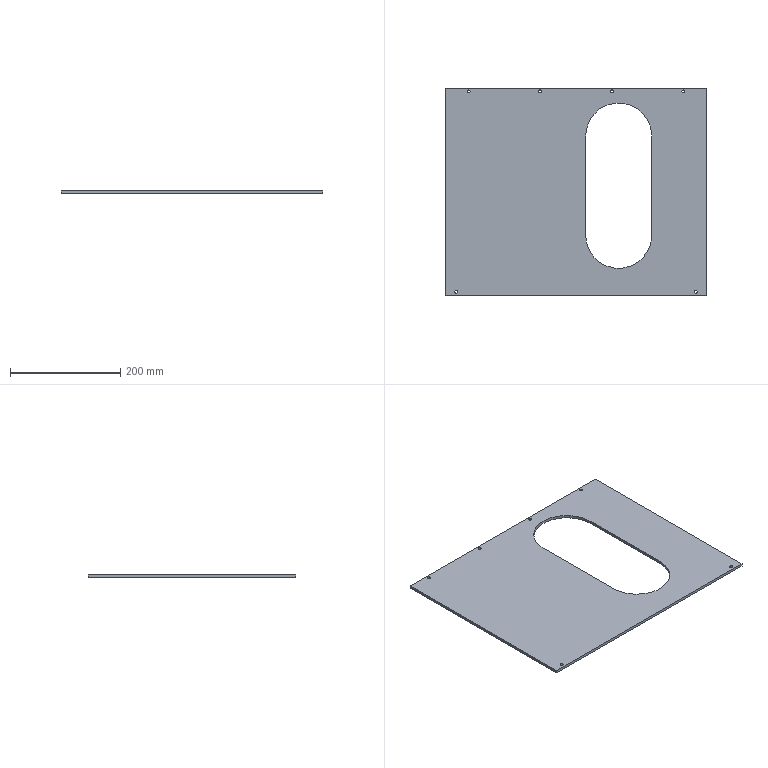Part | SolidWorks | features Extrusion 1, HoleWzd 1, ICE 1 | 1 solid | 22 faces | box 475 x 377 x 5 mm | volume 730114 mm3 | cylinder 14 | plane 8 | commonest cylinder face diameters 5.5 x12 120 x2
STEP:
#1=CARTESIAN_POINT('',(192.25,182.5,5.));
#2=VERTEX_POINT('',#1);
#3=CARTESIAN_POINT('',(197.75,182.5,5.));
#4=VERTEX_POINT('',#3);
#5=CARTESIAN_POINT('',(195.,182.5,5.));
#6=DIRECTION('',(0.,0.,1.));
#7=DIRECTION('',(1.,0.,0.));
#8=AXIS2_PLACEMENT_3D('',#5,#6,#7);
#9=CIRCLE('',#8,2.75);
#10=EDGE_CURVE('',#2,#4,#9,.T.);
#11=ORIENTED_EDGE('',*,*,#10,.T.);
#12=CARTESIAN_POINT('',(197.75,182.5,0.));
#13=VERTEX_POINT('',#12);
#14=CARTESIAN_POINT('',(197.75,182.5,0.));
#15=DIRECTION('',(0.,0.,-1.));
#16=VECTOR('',#15,1000.);
#17=LINE('',#14,#16);
#18=EDGE_CURVE('',#4,#13,#17,.T.);
#19=ORIENTED_EDGE('',*,*,#18,.T.);
#20=CARTESIAN_POINT('',(192.25,182.5,0.));
#21=VERTEX_POINT('',#20);
#22=CARTESIAN_POINT('',(195.,182.5,0.));
#23=DIRECTION('',(0.,0.,-1.));
#24=DIRECTION('',(-1.,0.,0.));
#25=AXIS2_PLACEMENT_3D('',#22,#23,#24);
#26=CIRCLE('',#25,2.75);
#27=EDGE_CURVE('',#13,#21,#26,.T.);
#28=ORIENTED_EDGE('',*,*,#27,.T.);
#29=CARTESIAN_POINT('',(192.25,182.5,0.));
#30=DIRECTION('',(0.,0.,-1.));
#31=VECTOR('',#30,1000.);
#32=LINE('',#29,#31);
#33=EDGE_CURVE('',#2,#21,#32,.T.);
#34=ORIENTED_EDGE('',*,*,#33,.F.);
#35=EDGE_LOOP('',(#11,#19,#28,#34));
#36=FACE_OUTER_BOUND('',#35,.T.);
#37=CARTESIAN_POINT('',(195.,182.5,0.));
#38=DIRECTION('',(0.,0.,-1.));
#39=DIRECTION('',(-1.,0.,0.));
#40=AXIS2_PLACEMENT_3D('',#37,#38,#39);
#41=CYLINDRICAL_SURFACE('',#40,2.75);
#42=ADVANCED_FACE('',(#36),#41,.F.);
#43=CARTESIAN_POINT('',(62.25,182.5,5.));
#44=VERTEX_POINT('',#43);
#45=CARTESIAN_POINT('',(67.75,182.5,5.));
#46=VERTEX_POINT('',#45);
#47=CARTESIAN_POINT('',(65.,182.5,5.));
#48=DIRECTION('',(0.,0.,1.));
#49=DIRECTION('',(1.,0.,0.));
#50=AXIS2_PLACEMENT_3D('',#47,#48,#49);
#51=CIRCLE('',#50,2.75);
#52=EDGE_CURVE('',#44,#46,#51,.T.);
#53=ORIENTED_EDGE('',*,*,#52,.T.);
#54=CARTESIAN_POINT('',(67.75,182.5,0.));
#55=VERTEX_POINT('',#54);
#56=CARTESIAN_POINT('',(67.75,182.5,0.));
#57=DIRECTION('',(0.,0.,-1.));
#58=VECTOR('',#57,1000.);
#59=LINE('',#56,#58);
#60=EDGE_CURVE('',#46,#55,#59,.T.);
#61=ORIENTED_EDGE('',*,*,#60,.T.);
#62=CARTESIAN_POINT('',(62.25,182.5,0.));
#63=VERTEX_POINT('',#62);
#64=CARTESIAN_POINT('',(65.,182.5,0.));
#65=DIRECTION('',(0.,0.,-1.));
#66=DIRECTION('',(-1.,0.,0.));
#67=AXIS2_PLACEMENT_3D('',#64,#65,#66);
#68=CIRCLE('',#67,2.75);
#69=EDGE_CURVE('',#55,#63,#68,.T.);
#70=ORIENTED_EDGE('',*,*,#69,.T.);
#71=CARTESIAN_POINT('',(62.25,182.5,0.));
#72=DIRECTION('',(0.,0.,-1.));
#73=VECTOR('',#72,1000.);
#74=LINE('',#71,#73);
#75=EDGE_CURVE('',#44,#63,#74,.T.);
#76=ORIENTED_EDGE('',*,*,#75,.F.);
#77=EDGE_LOOP('',(#53,#61,#70,#76));
#78=FACE_OUTER_BOUND('',#77,.T.);
#79=CARTESIAN_POINT('',(65.,182.5,0.));
#80=DIRECTION('',(0.,0.,-1.));
#81=DIRECTION('',(-1.,0.,0.));
#82=AXIS2_PLACEMENT_3D('',#79,#80,#81);
#83=CYLINDRICAL_SURFACE('',#82,2.75);
#84=ADVANCED_FACE('',(#78),#83,.F.);
#85=CARTESIAN_POINT('',(-67.75,182.5,5.));
#86=VERTEX_POINT('',#85);
#87=CARTESIAN_POINT('',(-62.25,182.5,5.));
#88=VERTEX_POINT('',#87);
#89=CARTESIAN_POINT('',(-65.,182.5,5.));
#90=DIRECTION('',(0.,0.,1.));
#91=DIRECTION('',(1.,0.,0.));
#92=AXIS2_PLACEMENT_3D('',#89,#90,#91);
#93=CIRCLE('',#92,2.75);
#94=EDGE_CURVE('',#86,#88,#93,.T.);
#95=ORIENTED_EDGE('',*,*,#94,.T.);
#96=CARTESIAN_POINT('',(-62.25,182.5,0.));
#97=VERTEX_POINT('',#96);
#98=CARTESIAN_POINT('',(-62.25,182.5,0.));
#99=DIRECTION('',(0.,0.,-1.));
#100=VECTOR('',#99,1000.);
#101=LINE('',#98,#100);
#102=EDGE_CURVE('',#88,#97,#101,.T.);
#103=ORIENTED_EDGE('',*,*,#102,.T.);
#104=CARTESIAN_POINT('',(-67.75,182.5,0.));
#105=VERTEX_POINT('',#104);
#106=CARTESIAN_POINT('',(-65.,182.5,0.));
#107=DIRECTION('',(0.,0.,-1.));
#108=DIRECTION('',(-1.,0.,0.));
#109=AXIS2_PLACEMENT_3D('',#106,#107,#108);
#110=CIRCLE('',#109,2.75);
#111=EDGE_CURVE('',#97,#105,#110,.T.);
#112=ORIENTED_EDGE('',*,*,#111,.T.);
#113=CARTESIAN_POINT('',(-67.75,182.5,0.));
#114=DIRECTION('',(0.,0.,-1.));
#115=VECTOR('',#114,1000.);
#116=LINE('',#113,#115);
#117=EDGE_CURVE('',#86,#105,#116,.T.);
#118=ORIENTED_EDGE('',*,*,#117,.F.);
#119=EDGE_LOOP('',(#95,#103,#112,#118));
#120=FACE_OUTER_BOUND('',#119,.T.);
#121=CARTESIAN_POINT('',(-65.,182.5,0.));
#122=DIRECTION('',(0.,0.,-1.));
#123=DIRECTION('',(-1.,0.,0.));
#124=AXIS2_PLACEMENT_3D('',#121,#122,#123);
#125=CYLINDRICAL_SURFACE('',#124,2.75);
#126=ADVANCED_FACE('',(#120),#125,.F.);
#127=CARTESIAN_POINT('',(-197.75,182.5,5.));
#128=VERTEX_POINT('',#127);
#129=CARTESIAN_POINT('',(-192.25,182.5,5.));
#130=VERTEX_POINT('',#129);
#131=CARTESIAN_POINT('',(-195.,182.5,5.));
#132=DIRECTION('',(0.,0.,1.));
#133=DIRECTION('',(1.,0.,0.));
#134=AXIS2_PLACEMENT_3D('',#131,#132,#133);
#135=CIRCLE('',#134,2.75);
#136=EDGE_CURVE('',#128,#130,#135,.T.);
#137=ORIENTED_EDGE('',*,*,#136,.T.);
#138=CARTESIAN_POINT('',(-192.25,182.5,0.));
#139=VERTEX_POINT('',#138);
#140=CARTESIAN_POINT('',(-192.25,182.5,0.));
#141=DIRECTION('',(0.,0.,-1.));
#142=VECTOR('',#141,1000.);
#143=LINE('',#140,#142);
#144=EDGE_CURVE('',#130,#139,#143,.T.);
#145=ORIENTED_EDGE('',*,*,#144,.T.);
#146=CARTESIAN_POINT('',(-197.75,182.5,0.));
#147=VERTEX_POINT('',#146);
#148=CARTESIAN_POINT('',(-195.,182.5,0.));
#149=DIRECTION('',(0.,0.,-1.));
#150=DIRECTION('',(-1.,0.,0.));
#151=AXIS2_PLACEMENT_3D('',#148,#149,#150);
#152=CIRCLE('',#151,2.75);
#153=EDGE_CURVE('',#139,#147,#152,.T.);
#154=ORIENTED_EDGE('',*,*,#153,.T.);
#155=CARTESIAN_POINT('',(-197.75,182.5,0.));
#156=DIRECTION('',(0.,0.,-1.));
#157=VECTOR('',#156,1000.);
#158=LINE('',#155,#157);
#159=EDGE_CURVE('',#128,#147,#158,.T.);
#160=ORIENTED_EDGE('',*,*,#159,.F.);
#161=EDGE_LOOP('',(#137,#145,#154,#160));
#162=FACE_OUTER_BOUND('',#161,.T.);
#163=CARTESIAN_POINT('',(-195.,182.5,0.));
#164=DIRECTION('',(0.,0.,-1.));
#165=DIRECTION('',(-1.,0.,0.));
#166=AXIS2_PLACEMENT_3D('',#163,#164,#165);
#167=CYLINDRICAL_SURFACE('',#166,2.75);
#168=ADVANCED_FACE('',(#162),#167,.F.);
#169=CARTESIAN_POINT('',(-220.25,-181.,5.));
#170=VERTEX_POINT('',#169);
#171=CARTESIAN_POINT('',(-214.75,-181.,5.));
#172=VERTEX_POINT('',#171);
#173=CARTESIAN_POINT('',(-217.5,-181.,5.));
#174=DIRECTION('',(0.,0.,1.));
#175=DIRECTION('',(1.,0.,0.));
#176=AXIS2_PLACEMENT_3D('',#173,#174,#175);
#177=CIRCLE('',#176,2.75);
#178=EDGE_CURVE('',#170,#172,#177,.T.);
#179=ORIENTED_EDGE('',*,*,#178,.T.);
#180=CARTESIAN_POINT('',(-214.75,-181.,0.));
#181=VERTEX_POINT('',#180);
#182=CARTESIAN_POINT('',(-214.75,-181.,0.));
#183=DIRECTION('',(0.,0.,-1.));
#184=VECTOR('',#183,1000.);
#185=LINE('',#182,#184);
#186=EDGE_CURVE('',#172,#181,#185,.T.);
#187=ORIENTED_EDGE('',*,*,#186,.T.);
#188=CARTESIAN_POINT('',(-220.25,-181.,0.));
#189=VERTEX_POINT('',#188);
#190=CARTESIAN_POINT('',(-217.5,-181.,0.));
#191=DIRECTION('',(0.,0.,-1.));
#192=DIRECTION('',(-1.,0.,0.));
#193=AXIS2_PLACEMENT_3D('',#190,#191,#192);
#194=CIRCLE('',#193,2.75);
#195=EDGE_CURVE('',#181,#189,#194,.T.);
#196=ORIENTED_EDGE('',*,*,#195,.T.);
#197=CARTESIAN_POINT('',(-220.25,-181.,0.));
#198=DIRECTION('',(0.,0.,-1.));
#199=VECTOR('',#198,1000.);
#200=LINE('',#197,#199);
#201=EDGE_CURVE('',#170,#189,#200,.T.);
#202=ORIENTED_EDGE('',*,*,#201,.F.);
#203=EDGE_LOOP('',(#179,#187,#196,#202));
#204=FACE_OUTER_BOUND('',#203,.T.);
#205=CARTESIAN_POINT('',(-217.5,-181.,0.));
#206=DIRECTION('',(0.,0.,-1.));
#207=DIRECTION('',(-1.,0.,0.));
#208=AXIS2_PLACEMENT_3D('',#205,#206,#207);
#209=CYLINDRICAL_SURFACE('',#208,2.75);
#210=ADVANCED_FACE('',(#204),#209,.F.);
#211=CARTESIAN_POINT('',(214.75,-181.,5.));
#212=VERTEX_POINT('',#211);
#213=CARTESIAN_POINT('',(220.25,-181.,5.));
#214=VERTEX_POINT('',#213);
#215=CARTESIAN_POINT('',(217.5,-181.,5.));
#216=DIRECTION('',(0.,0.,1.));
#217=DIRECTION('',(1.,0.,0.));
#218=AXIS2_PLACEMENT_3D('',#215,#216,#217);
#219=CIRCLE('',#218,2.75);
#220=EDGE_CURVE('',#212,#214,#219,.T.);
#221=ORIENTED_EDGE('',*,*,#220,.T.);
#222=CARTESIAN_POINT('',(220.25,-181.,0.));
#223=VERTEX_POINT('',#222);
#224=CARTESIAN_POINT('',(220.25,-181.,0.));
#225=DIRECTION('',(0.,0.,-1.));
#226=VECTOR('',#225,1000.);
#227=LINE('',#224,#226);
#228=EDGE_CURVE('',#214,#223,#227,.T.);
#229=ORIENTED_EDGE('',*,*,#228,.T.);
#230=CARTESIAN_POINT('',(214.75,-181.,0.));
#231=VERTEX_POINT('',#230);
#232=CARTESIAN_POINT('',(217.5,-181.,0.));
#233=DIRECTION('',(0.,0.,-1.));
#234=DIRECTION('',(-1.,0.,0.));
#235=AXIS2_PLACEMENT_3D('',#232,#233,#234);
#236=CIRCLE('',#235,2.75);
#237=EDGE_CURVE('',#223,#231,#236,.T.);
#238=ORIENTED_EDGE('',*,*,#237,.T.);
#239=CARTESIAN_POINT('',(214.75,-181.,0.));
#240=DIRECTION('',(0.,0.,-1.));
#241=VECTOR('',#240,1000.);
#242=LINE('',#239,#241);
#243=EDGE_CURVE('',#212,#231,#242,.T.);
#244=ORIENTED_EDGE('',*,*,#243,.F.);
#245=EDGE_LOOP('',(#221,#229,#238,#244));
#246=FACE_OUTER_BOUND('',#245,.T.);
#247=CARTESIAN_POINT('',(217.5,-181.,0.));
#248=DIRECTION('',(0.,0.,-1.));
#249=DIRECTION('',(-1.,0.,0.));
#250=AXIS2_PLACEMENT_3D('',#247,#248,#249);
#251=CYLINDRICAL_SURFACE('',#250,2.75);
#252=ADVANCED_FACE('',(#246),#251,.F.);
#253=CARTESIAN_POINT('',(137.5,101.5,0.));
#254=VERTEX_POINT('',#253);
#255=CARTESIAN_POINT('',(137.5,-78.5,0.));
#256=VERTEX_POINT('',#255);
#257=CARTESIAN_POINT('',(137.5,101.5,0.));
#258=DIRECTION('',(0.,-1.,0.));
#259=VECTOR('',#258,1000.);
#260=LINE('',#257,#259);
#261=EDGE_CURVE('',#254,#256,#260,.T.);
#262=ORIENTED_EDGE('',*,*,#261,.F.);
#263=CARTESIAN_POINT('',(17.5,101.5,0.));
#264=VERTEX_POINT('',#263);
#265=CARTESIAN_POINT('',(77.5,101.5,0.));
#266=DIRECTION('',(0.,0.,-1.));
#267=DIRECTION('',(-1.,0.,0.));
#268=AXIS2_PLACEMENT_3D('',#265,#266,#267);
#269=CIRCLE('',#268,60.);
#270=EDGE_CURVE('',#264,#254,#269,.T.);
#271=ORIENTED_EDGE('',*,*,#270,.F.);
#272=CARTESIAN_POINT('',(17.5,-78.5,0.));
#273=VERTEX_POINT('',#272);
#274=CARTESIAN_POINT('',(17.5,101.5,0.));
#275=DIRECTION('',(0.,1.,0.));
#276=VECTOR('',#275,1000.);
#277=LINE('',#274,#276);
#278=EDGE_CURVE('',#273,#264,#277,.T.);
#279=ORIENTED_EDGE('',*,*,#278,.F.);
#280=CARTESIAN_POINT('',(77.5,-78.5,0.));
#281=DIRECTION('',(0.,0.,-1.));
#282=DIRECTION('',(-1.,0.,0.));
#283=AXIS2_PLACEMENT_3D('',#280,#281,#282);
#284=CIRCLE('',#283,60.);
#285=EDGE_CURVE('',#256,#273,#284,.T.);
#286=ORIENTED_EDGE('',*,*,#285,.F.);
#287=EDGE_LOOP('',(#262,#271,#279,#286));
#288=FACE_BOUND('',#287,.T.);
#289=CARTESIAN_POINT('',(195.,182.5,0.));
#290=DIRECTION('',(0.,0.,-1.));
#291=DIRECTION('',(-1.,0.,0.));
#292=AXIS2_PLACEMENT_3D('',#289,#290,#291);
#293=CIRCLE('',#292,2.75);
#294=EDGE_CURVE('',#21,#13,#293,.T.);
#295=ORIENTED_EDGE('',*,*,#294,.F.);
#296=ORIENTED_EDGE('',*,*,#27,.F.);
#297=EDGE_LOOP('',(#295,#296));
#298=FACE_BOUND('',#297,.T.);
#299=CARTESIAN_POINT('',(65.,182.5,0.));
#300=DIRECTION('',(0.,0.,-1.));
#301=DIRECTION('',(-1.,0.,0.));
#302=AXIS2_PLACEMENT_3D('',#299,#300,#301);
#303=CIRCLE('',#302,2.75);
#304=EDGE_CURVE('',#63,#55,#303,.T.);
#305=ORIENTED_EDGE('',*,*,#304,.F.);
#306=ORIENTED_EDGE('',*,*,#69,.F.);
#307=EDGE_LOOP('',(#305,#306));
#308=FACE_BOUND('',#307,.T.);
#309=CARTESIAN_POINT('',(-195.,182.5,0.));
#310=DIRECTION('',(0.,0.,-1.));
#311=DIRECTION('',(-1.,0.,0.));
#312=AXIS2_PLACEMENT_3D('',#309,#310,#311);
#313=CIRCLE('',#312,2.75);
#314=EDGE_CURVE('',#147,#139,#313,.T.);
#315=ORIENTED_EDGE('',*,*,#314,.F.);
#316=ORIENTED_EDGE('',*,*,#153,.F.);
#317=EDGE_LOOP('',(#315,#316));
#318=FACE_BOUND('',#317,.T.);
#319=CARTESIAN_POINT('',(-217.5,-181.,0.));
#320=DIRECTION('',(0.,0.,-1.));
#321=DIRECTION('',(-1.,0.,0.));
#322=AXIS2_PLACEMENT_3D('',#319,#320,#321);
#323=CIRCLE('',#322,2.75);
#324=EDGE_CURVE('',#189,#181,#323,.T.);
#325=ORIENTED_EDGE('',*,*,#324,.F.);
#326=ORIENTED_EDGE('',*,*,#195,.F.);
#327=EDGE_LOOP('',(#325,#326));
#328=FACE_BOUND('',#327,.T.);
#329=CARTESIAN_POINT('',(217.5,-181.,0.));
#330=DIRECTION('',(0.,0.,-1.));
#331=DIRECTION('',(-1.,0.,0.));
#332=AXIS2_PLACEMENT_3D('',#329,#330,#331);
#333=CIRCLE('',#332,2.75);
#334=EDGE_CURVE('',#231,#223,#333,.T.);
#335=ORIENTED_EDGE('',*,*,#334,.F.);
#336=ORIENTED_EDGE('',*,*,#237,.F.);
#337=EDGE_LOOP('',(#335,#336));
#338=FACE_BOUND('',#337,.T.);
#339=CARTESIAN_POINT('',(237.5,-188.5,0.));
#340=VERTEX_POINT('',#339);
#341=CARTESIAN_POINT('',(237.5,188.5,0.));
#342=VERTEX_POINT('',#341);
#343=CARTESIAN_POINT('',(237.5,188.5,0.));
#344=DIRECTION('',(0.,1.,0.));
#345=VECTOR('',#344,1000.);
#346=LINE('',#343,#345);
#347=EDGE_CURVE('',#340,#342,#346,.T.);
#348=ORIENTED_EDGE('',*,*,#347,.F.);
#349=CARTESIAN_POINT('',(-237.5,-188.5,0.));
#350=VERTEX_POINT('',#349);
#351=CARTESIAN_POINT('',(-237.5,-188.5,0.));
#352=DIRECTION('',(1.,0.,0.));
#353=VECTOR('',#352,1000.);
#354=LINE('',#351,#353);
#355=EDGE_CURVE('',#350,#340,#354,.T.);
#356=ORIENTED_EDGE('',*,*,#355,.F.);
#357=CARTESIAN_POINT('',(-237.5,188.5,0.));
#358=VERTEX_POINT('',#357);
#359=CARTESIAN_POINT('',(-237.5,188.5,0.));
#360=DIRECTION('',(0.,-1.,0.));
#361=VECTOR('',#360,1000.);
#362=LINE('',#359,#361);
#363=EDGE_CURVE('',#358,#350,#362,.T.);
#364=ORIENTED_EDGE('',*,*,#363,.F.);
#365=CARTESIAN_POINT('',(-237.5,188.5,0.));
#366=DIRECTION('',(-1.,0.,0.));
#367=VECTOR('',#366,1000.);
#368=LINE('',#365,#367);
#369=EDGE_CURVE('',#342,#358,#368,.T.);
#370=ORIENTED_EDGE('',*,*,#369,.F.);
#371=EDGE_LOOP('',(#348,#356,#364,#370));
#372=FACE_OUTER_BOUND('',#371,.T.);
#373=CARTESIAN_POINT('',(-65.,182.5,0.));
#374=DIRECTION('',(0.,0.,-1.));
#375=DIRECTION('',(-1.,0.,0.));
#376=AXIS2_PLACEMENT_3D('',#373,#374,#375);
#377=CIRCLE('',#376,2.75);
#378=EDGE_CURVE('',#105,#97,#377,.T.);
#379=ORIENTED_EDGE('',*,*,#378,.F.);
#380=ORIENTED_EDGE('',*,*,#111,.F.);
#381=EDGE_LOOP('',(#379,#380));
#382=FACE_BOUND('',#381,.T.);
#383=CARTESIAN_POINT('',(0.,0.,0.));
#384=DIRECTION('',(0.,0.,1.));
#385=DIRECTION('',(1.,0.,0.));
#386=AXIS2_PLACEMENT_3D('',#383,#384,#385);
#387=PLANE('',#386);
#388=ADVANCED_FACE('',(#288,#298,#308,#318,#328,#338,#372,#382),#387,.F.);
#389=ORIENTED_EDGE('',*,*,#347,.T.);
#390=CARTESIAN_POINT('',(237.5,188.5,5.));
#391=VERTEX_POINT('',#390);
#392=CARTESIAN_POINT('',(237.5,188.5,5.));
#393=DIRECTION('',(0.,0.,-1.));
#394=VECTOR('',#393,1000.);
#395=LINE('',#392,#394);
#396=EDGE_CURVE('',#391,#342,#395,.T.);
#397=ORIENTED_EDGE('',*,*,#396,.F.);
#398=CARTESIAN_POINT('',(237.5,-188.5,5.));
#399=VERTEX_POINT('',#398);
#400=CARTESIAN_POINT('',(237.5,188.5,5.));
#401=DIRECTION('',(0.,1.,0.));
#402=VECTOR('',#401,1000.);
#403=LINE('',#400,#402);
#404=EDGE_CURVE('',#399,#391,#403,.T.);
#405=ORIENTED_EDGE('',*,*,#404,.F.);
#406=CARTESIAN_POINT('',(237.5,-188.5,5.));
#407=DIRECTION('',(0.,0.,-1.));
#408=VECTOR('',#407,1000.);
#409=LINE('',#406,#408);
#410=EDGE_CURVE('',#399,#340,#409,.T.);
#411=ORIENTED_EDGE('',*,*,#410,.T.);
#412=EDGE_LOOP('',(#389,#397,#405,#411));
#413=FACE_OUTER_BOUND('',#412,.T.);
#414=CARTESIAN_POINT('',(237.5,188.5,5.));
#415=DIRECTION('',(-1.,0.,0.));
#416=DIRECTION('',(0.,-1.,0.));
#417=AXIS2_PLACEMENT_3D('',#414,#415,#416);
#418=PLANE('',#417);
#419=ADVANCED_FACE('',(#413),#418,.F.);
#420=ORIENTED_EDGE('',*,*,#369,.T.);
#421=CARTESIAN_POINT('',(-237.5,188.5,5.));
#422=VERTEX_POINT('',#421);
#423=CARTESIAN_POINT('',(-237.5,188.5,5.));
#424=DIRECTION('',(0.,0.,-1.));
#425=VECTOR('',#424,1000.);
#426=LINE('',#423,#425);
#427=EDGE_CURVE('',#422,#358,#426,.T.);
#428=ORIENTED_EDGE('',*,*,#427,.F.);
#429=CARTESIAN_POINT('',(-237.5,188.5,5.));
#430=DIRECTION('',(-1.,0.,0.));
#431=VECTOR('',#430,1000.);
#432=LINE('',#429,#431);
#433=EDGE_CURVE('',#391,#422,#432,.T.);
#434=ORIENTED_EDGE('',*,*,#433,.F.);
#435=ORIENTED_EDGE('',*,*,#396,.T.);
#436=EDGE_LOOP('',(#420,#428,#434,#435));
#437=FACE_OUTER_BOUND('',#436,.T.);
#438=CARTESIAN_POINT('',(-237.5,188.5,5.));
#439=DIRECTION('',(0.,-1.,0.));
#440=DIRECTION('',(0.,0.,-1.));
#441=AXIS2_PLACEMENT_3D('',#438,#439,#440);
#442=PLANE('',#441);
#443=ADVANCED_FACE('',(#437),#442,.F.);
#444=ORIENTED_EDGE('',*,*,#363,.T.);
#445=CARTESIAN_POINT('',(-237.5,-188.5,5.));
#446=VERTEX_POINT('',#445);
#447=CARTESIAN_POINT('',(-237.5,-188.5,5.));
#448=DIRECTION('',(0.,0.,-1.));
#449=VECTOR('',#448,1000.);
#450=LINE('',#447,#449);
#451=EDGE_CURVE('',#446,#350,#450,.T.);
#452=ORIENTED_EDGE('',*,*,#451,.F.);
#453=CARTESIAN_POINT('',(-237.5,188.5,5.));
#454=DIRECTION('',(0.,-1.,0.));
#455=VECTOR('',#454,1000.);
#456=LINE('',#453,#455);
#457=EDGE_CURVE('',#422,#446,#456,.T.);
#458=ORIENTED_EDGE('',*,*,#457,.F.);
#459=ORIENTED_EDGE('',*,*,#427,.T.);
#460=EDGE_LOOP('',(#444,#452,#458,#459));
#461=FACE_OUTER_BOUND('',#460,.T.);
#462=CARTESIAN_POINT('',(-237.5,188.5,5.));
#463=DIRECTION('',(1.,0.,0.));
#464=DIRECTION('',(0.,0.,-1.));
#465=AXIS2_PLACEMENT_3D('',#462,#463,#464);
#466=PLANE('',#465);
#467=ADVANCED_FACE('',(#461),#466,.F.);
#468=ORIENTED_EDGE('',*,*,#355,.T.);
#469=ORIENTED_EDGE('',*,*,#410,.F.);
#470=CARTESIAN_POINT('',(-237.5,-188.5,5.));
#471=DIRECTION('',(1.,0.,0.));
#472=VECTOR('',#471,1000.);
#473=LINE('',#470,#472);
#474=EDGE_CURVE('',#446,#399,#473,.T.);
#475=ORIENTED_EDGE('',*,*,#474,.F.);
#476=ORIENTED_EDGE('',*,*,#451,.T.);
#477=EDGE_LOOP('',(#468,#469,#475,#476));
#478=FACE_OUTER_BOUND('',#477,.T.);
#479=CARTESIAN_POINT('',(-237.5,-188.5,5.));
#480=DIRECTION('',(0.,1.,0.));
#481=DIRECTION('',(0.,0.,1.));
#482=AXIS2_PLACEMENT_3D('',#479,#480,#481);
#483=PLANE('',#482);
#484=ADVANCED_FACE('',(#478),#483,.F.);
#485=CARTESIAN_POINT('',(137.5,101.5,5.));
#486=VERTEX_POINT('',#485);
#487=CARTESIAN_POINT('',(17.5,101.5,5.));
#488=VERTEX_POINT('',#487);
#489=CARTESIAN_POINT('',(77.5,101.5,5.));
#490=DIRECTION('',(0.,0.,1.));
#491=DIRECTION('',(1.,0.,0.));
#492=AXIS2_PLACEMENT_3D('',#489,#490,#491);
#493=CIRCLE('',#492,60.);
#494=EDGE_CURVE('',#486,#488,#493,.T.);
#495=ORIENTED_EDGE('',*,*,#494,.F.);
#496=CARTESIAN_POINT('',(137.5,-78.5,5.));
#497=VERTEX_POINT('',#496);
#498=CARTESIAN_POINT('',(137.5,0.,5.));
#499=DIRECTION('',(0.,1.,0.));
#500=VECTOR('',#499,1000.);
#501=LINE('',#498,#500);
#502=EDGE_CURVE('',#497,#486,#501,.T.);
#503=ORIENTED_EDGE('',*,*,#502,.F.);
#504=CARTESIAN_POINT('',(17.5,-78.5,5.));
#505=VERTEX_POINT('',#504);
#506=CARTESIAN_POINT('',(77.5,-78.5,5.));
#507=DIRECTION('',(0.,0.,1.));
#508=DIRECTION('',(1.,0.,0.));
#509=AXIS2_PLACEMENT_3D('',#506,#507,#508);
#510=CIRCLE('',#509,60.);
#511=EDGE_CURVE('',#505,#497,#510,.T.);
#512=ORIENTED_EDGE('',*,*,#511,.F.);
#513=CARTESIAN_POINT('',(17.5,0.,5.));
#514=DIRECTION('',(0.,-1.,0.));
#515=VECTOR('',#514,1000.);
#516=LINE('',#513,#515);
#517=EDGE_CURVE('',#488,#505,#516,.T.);
#518=ORIENTED_EDGE('',*,*,#517,.F.);
#519=EDGE_LOOP('',(#495,#503,#512,#518));
#520=FACE_BOUND('',#519,.T.);
#521=ORIENTED_EDGE('',*,*,#10,.F.);
#522=CARTESIAN_POINT('',(195.,182.5,5.));
#523=DIRECTION('',(0.,0.,1.));
#524=DIRECTION('',(1.,0.,0.));
#525=AXIS2_PLACEMENT_3D('',#522,#523,#524);
#526=CIRCLE('',#525,2.75);
#527=EDGE_CURVE('',#4,#2,#526,.T.);
#528=ORIENTED_EDGE('',*,*,#527,.F.);
#529=EDGE_LOOP('',(#521,#528));
#530=FACE_BOUND('',#529,.T.);
#531=ORIENTED_EDGE('',*,*,#52,.F.);
#532=CARTESIAN_POINT('',(65.,182.5,5.));
#533=DIRECTION('',(0.,0.,1.));
#534=DIRECTION('',(1.,0.,0.));
#535=AXIS2_PLACEMENT_3D('',#532,#533,#534);
#536=CIRCLE('',#535,2.75);
#537=EDGE_CURVE('',#46,#44,#536,.T.);
#538=ORIENTED_EDGE('',*,*,#537,.F.);
#539=EDGE_LOOP('',(#531,#538));
#540=FACE_BOUND('',#539,.T.);
#541=ORIENTED_EDGE('',*,*,#94,.F.);
#542=CARTESIAN_POINT('',(-65.,182.5,5.));
#543=DIRECTION('',(0.,0.,1.));
#544=DIRECTION('',(1.,0.,0.));
#545=AXIS2_PLACEMENT_3D('',#542,#543,#544);
#546=CIRCLE('',#545,2.75);
#547=EDGE_CURVE('',#88,#86,#546,.T.);
#548=ORIENTED_EDGE('',*,*,#547,.F.);
#549=EDGE_LOOP('',(#541,#548));
#550=FACE_BOUND('',#549,.T.);
#551=ORIENTED_EDGE('',*,*,#136,.F.);
#552=CARTESIAN_POINT('',(-195.,182.5,5.));
#553=DIRECTION('',(0.,0.,1.));
#554=DIRECTION('',(1.,0.,0.));
#555=AXIS2_PLACEMENT_3D('',#552,#553,#554);
#556=CIRCLE('',#555,2.75);
#557=EDGE_CURVE('',#130,#128,#556,.T.);
#558=ORIENTED_EDGE('',*,*,#557,.F.);
#559=EDGE_LOOP('',(#551,#558));
#560=FACE_BOUND('',#559,.T.);
#561=ORIENTED_EDGE('',*,*,#178,.F.);
#562=CARTESIAN_POINT('',(-217.5,-181.,5.));
#563=DIRECTION('',(0.,0.,1.));
#564=DIRECTION('',(1.,0.,0.));
#565=AXIS2_PLACEMENT_3D('',#562,#563,#564);
#566=CIRCLE('',#565,2.75);
#567=EDGE_CURVE('',#172,#170,#566,.T.);
#568=ORIENTED_EDGE('',*,*,#567,.F.);
#569=EDGE_LOOP('',(#561,#568));
#570=FACE_BOUND('',#569,.T.);
#571=ORIENTED_EDGE('',*,*,#220,.F.);
#572=CARTESIAN_POINT('',(217.5,-181.,5.));
#573=DIRECTION('',(0.,0.,1.));
#574=DIRECTION('',(1.,0.,0.));
#575=AXIS2_PLACEMENT_3D('',#572,#573,#574);
#576=CIRCLE('',#575,2.75);
#577=EDGE_CURVE('',#214,#212,#576,.T.);
#578=ORIENTED_EDGE('',*,*,#577,.F.);
#579=EDGE_LOOP('',(#571,#578));
#580=FACE_BOUND('',#579,.T.);
#581=ORIENTED_EDGE('',*,*,#404,.T.);
#582=ORIENTED_EDGE('',*,*,#433,.T.);
#583=ORIENTED_EDGE('',*,*,#457,.T.);
#584=ORIENTED_EDGE('',*,*,#474,.T.);
#585=EDGE_LOOP('',(#581,#582,#583,#584));
#586=FACE_OUTER_BOUND('',#585,.T.);
#587=CARTESIAN_POINT('',(0.,0.,5.));
#588=DIRECTION('',(0.,0.,1.));
#589=DIRECTION('',(1.,0.,0.));
#590=AXIS2_PLACEMENT_3D('',#587,#588,#589);
#591=PLANE('',#590);
#592=ADVANCED_FACE('',(#520,#530,#540,#550,#560,#570,#580,#586),#591,.T.);
#593=ORIENTED_EDGE('',*,*,#228,.F.);
#594=ORIENTED_EDGE('',*,*,#577,.T.);
#595=ORIENTED_EDGE('',*,*,#243,.T.);
#596=ORIENTED_EDGE('',*,*,#334,.T.);
#597=EDGE_LOOP('',(#593,#594,#595,#596));
#598=FACE_OUTER_BOUND('',#597,.T.);
#599=CARTESIAN_POINT('',(217.5,-181.,0.));
#600=DIRECTION('',(0.,0.,-1.));
#601=DIRECTION('',(-1.,0.,0.));
#602=AXIS2_PLACEMENT_3D('',#599,#600,#601);
#603=CYLINDRICAL_SURFACE('',#602,2.75);
#604=ADVANCED_FACE('',(#598),#603,.F.);
#605=ORIENTED_EDGE('',*,*,#186,.F.);
#606=ORIENTED_EDGE('',*,*,#567,.T.);
#607=ORIENTED_EDGE('',*,*,#201,.T.);
#608=ORIENTED_EDGE('',*,*,#324,.T.);
#609=EDGE_LOOP('',(#605,#606,#607,#608));
#610=FACE_OUTER_BOUND('',#609,.T.);
#611=CARTESIAN_POINT('',(-217.5,-181.,0.));
#612=DIRECTION('',(0.,0.,-1.));
#613=DIRECTION('',(-1.,0.,0.));
#614=AXIS2_PLACEMENT_3D('',#611,#612,#613);
#615=CYLINDRICAL_SURFACE('',#614,2.75);
#616=ADVANCED_FACE('',(#610),#615,.F.);
#617=ORIENTED_EDGE('',*,*,#144,.F.);
#618=ORIENTED_EDGE('',*,*,#557,.T.);
#619=ORIENTED_EDGE('',*,*,#159,.T.);
#620=ORIENTED_EDGE('',*,*,#314,.T.);
#621=EDGE_LOOP('',(#617,#618,#619,#620));
#622=FACE_OUTER_BOUND('',#621,.T.);
#623=CARTESIAN_POINT('',(-195.,182.5,0.));
#624=DIRECTION('',(0.,0.,-1.));
#625=DIRECTION('',(-1.,0.,0.));
#626=AXIS2_PLACEMENT_3D('',#623,#624,#625);
#627=CYLINDRICAL_SURFACE('',#626,2.75);
#628=ADVANCED_FACE('',(#622),#627,.F.);
#629=ORIENTED_EDGE('',*,*,#102,.F.);
#630=ORIENTED_EDGE('',*,*,#547,.T.);
#631=ORIENTED_EDGE('',*,*,#117,.T.);
#632=ORIENTED_EDGE('',*,*,#378,.T.);
#633=EDGE_LOOP('',(#629,#630,#631,#632));
#634=FACE_OUTER_BOUND('',#633,.T.);
#635=CARTESIAN_POINT('',(-65.,182.5,0.));
#636=DIRECTION('',(0.,0.,-1.));
#637=DIRECTION('',(-1.,0.,0.));
#638=AXIS2_PLACEMENT_3D('',#635,#636,#637);
#639=CYLINDRICAL_SURFACE('',#638,2.75);
#640=ADVANCED_FACE('',(#634),#639,.F.);
#641=ORIENTED_EDGE('',*,*,#60,.F.);
#642=ORIENTED_EDGE('',*,*,#537,.T.);
#643=ORIENTED_EDGE('',*,*,#75,.T.);
#644=ORIENTED_EDGE('',*,*,#304,.T.);
#645=EDGE_LOOP('',(#641,#642,#643,#644));
#646=FACE_OUTER_BOUND('',#645,.T.);
#647=CARTESIAN_POINT('',(65.,182.5,0.));
#648=DIRECTION('',(0.,0.,-1.));
#649=DIRECTION('',(-1.,0.,0.));
#650=AXIS2_PLACEMENT_3D('',#647,#648,#649);
#651=CYLINDRICAL_SURFACE('',#650,2.75);
#652=ADVANCED_FACE('',(#646),#651,.F.);
#653=ORIENTED_EDGE('',*,*,#18,.F.);
#654=ORIENTED_EDGE('',*,*,#527,.T.);
#655=ORIENTED_EDGE('',*,*,#33,.T.);
#656=ORIENTED_EDGE('',*,*,#294,.T.);
#657=EDGE_LOOP('',(#653,#654,#655,#656));
#658=FACE_OUTER_BOUND('',#657,.T.);
#659=CARTESIAN_POINT('',(195.,182.5,0.));
#660=DIRECTION('',(0.,0.,-1.));
#661=DIRECTION('',(-1.,0.,0.));
#662=AXIS2_PLACEMENT_3D('',#659,#660,#661);
#663=CYLINDRICAL_SURFACE('',#662,2.75);
#664=ADVANCED_FACE('',(#658),#663,.F.);
#665=ORIENTED_EDGE('',*,*,#494,.T.);
#666=CARTESIAN_POINT('',(17.5,101.5,10.));
#667=DIRECTION('',(0.,0.,-1.));
#668=VECTOR('',#667,1000.);
#669=LINE('',#666,#668);
#670=EDGE_CURVE('',#488,#264,#669,.T.);
#671=ORIENTED_EDGE('',*,*,#670,.T.);
#672=ORIENTED_EDGE('',*,*,#270,.T.);
#673=CARTESIAN_POINT('',(137.5,101.5,10.));
#674=DIRECTION('',(0.,0.,-1.));
#675=VECTOR('',#674,1000.);
#676=LINE('',#673,#675);
#677=EDGE_CURVE('',#486,#254,#676,.T.);
#678=ORIENTED_EDGE('',*,*,#677,.F.);
#679=EDGE_LOOP('',(#665,#671,#672,#678));
#680=FACE_OUTER_BOUND('',#679,.T.);
#681=CARTESIAN_POINT('',(77.5,101.5,10.));
#682=DIRECTION('',(0.,0.,-1.));
#683=DIRECTION('',(-1.,0.,0.));
#684=AXIS2_PLACEMENT_3D('',#681,#682,#683);
#685=CYLINDRICAL_SURFACE('',#684,60.);
#686=ADVANCED_FACE('',(#680),#685,.F.);
#687=ORIENTED_EDGE('',*,*,#517,.T.);
#688=CARTESIAN_POINT('',(17.5,-78.5,10.));
#689=DIRECTION('',(0.,0.,-1.));
#690=VECTOR('',#689,1000.);
#691=LINE('',#688,#690);
#692=EDGE_CURVE('',#505,#273,#691,.T.);
#693=ORIENTED_EDGE('',*,*,#692,.T.);
#694=ORIENTED_EDGE('',*,*,#278,.T.);
#695=ORIENTED_EDGE('',*,*,#670,.F.);
#696=EDGE_LOOP('',(#687,#693,#694,#695));
#697=FACE_OUTER_BOUND('',#696,.T.);
#698=CARTESIAN_POINT('',(17.5,101.5,10.));
#699=DIRECTION('',(-1.,0.,0.));
#700=DIRECTION('',(0.,-1.,0.));
#701=AXIS2_PLACEMENT_3D('',#698,#699,#700);
#702=PLANE('',#701);
#703=ADVANCED_FACE('',(#697),#702,.F.);
#704=ORIENTED_EDGE('',*,*,#511,.T.);
#705=CARTESIAN_POINT('',(137.5,-78.5,10.));
#706=DIRECTION('',(0.,0.,-1.));
#707=VECTOR('',#706,1000.);
#708=LINE('',#705,#707);
#709=EDGE_CURVE('',#497,#256,#708,.T.);
#710=ORIENTED_EDGE('',*,*,#709,.T.);
#711=ORIENTED_EDGE('',*,*,#285,.T.);
#712=ORIENTED_EDGE('',*,*,#692,.F.);
#713=EDGE_LOOP('',(#704,#710,#711,#712));
#714=FACE_OUTER_BOUND('',#713,.T.);
#715=CARTESIAN_POINT('',(77.5,-78.5,10.));
#716=DIRECTION('',(0.,0.,-1.));
#717=DIRECTION('',(-1.,0.,0.));
#718=AXIS2_PLACEMENT_3D('',#715,#716,#717);
#719=CYLINDRICAL_SURFACE('',#718,60.);
#720=ADVANCED_FACE('',(#714),#719,.F.);
#721=ORIENTED_EDGE('',*,*,#502,.T.);
#722=ORIENTED_EDGE('',*,*,#677,.T.);
#723=ORIENTED_EDGE('',*,*,#261,.T.);
#724=ORIENTED_EDGE('',*,*,#709,.F.);
#725=EDGE_LOOP('',(#721,#722,#723,#724));
#726=FACE_OUTER_BOUND('',#725,.T.);
#727=CARTESIAN_POINT('',(137.5,101.5,10.));
#728=DIRECTION('',(1.,0.,0.));
#729=DIRECTION('',(0.,1.,0.));
#730=AXIS2_PLACEMENT_3D('',#727,#728,#729);
#731=PLANE('',#730);
#732=ADVANCED_FACE('',(#726),#731,.F.);
#733=CLOSED_SHELL('',(#42,#84,#126,#168,#210,#252,#388,#419,#443,#467,#484,#592,#604,#616,#628,#640,#652,#664,#686,#703,#720,#732));
#734=MANIFOLD_SOLID_BREP('',#733);
#735=CARTESIAN_POINT('',(0.,0.,0.));
#736=DIRECTION('',(0.,0.,1.));
#737=DIRECTION('',(1.,0.,0.));
#738=AXIS2_PLACEMENT_3D('',#735,#736,#737);
#739=(LENGTH_UNIT()NAMED_UNIT(*)SI_UNIT(.MILLI.,.METRE.));
#740=UNCERTAINTY_MEASURE_WITH_UNIT(LENGTH_MEASURE(0.00001),#739,'','');
#741=(NAMED_UNIT(*)PLANE_ANGLE_UNIT()SI_UNIT($,.RADIAN.));
#742=(NAMED_UNIT(*)SI_UNIT($,.STERADIAN.)SOLID_ANGLE_UNIT());
#743=(GEOMETRIC_REPRESENTATION_CONTEXT(3)GLOBAL_UNCERTAINTY_ASSIGNED_CONTEXT((#740))GLOBAL_UNIT_ASSIGNED_CONTEXT((#739,#741,#742))REPRESENTATION_CONTEXT('',''));
#744=ADVANCED_BREP_SHAPE_REPRESENTATION('',(#734,#738),#743);